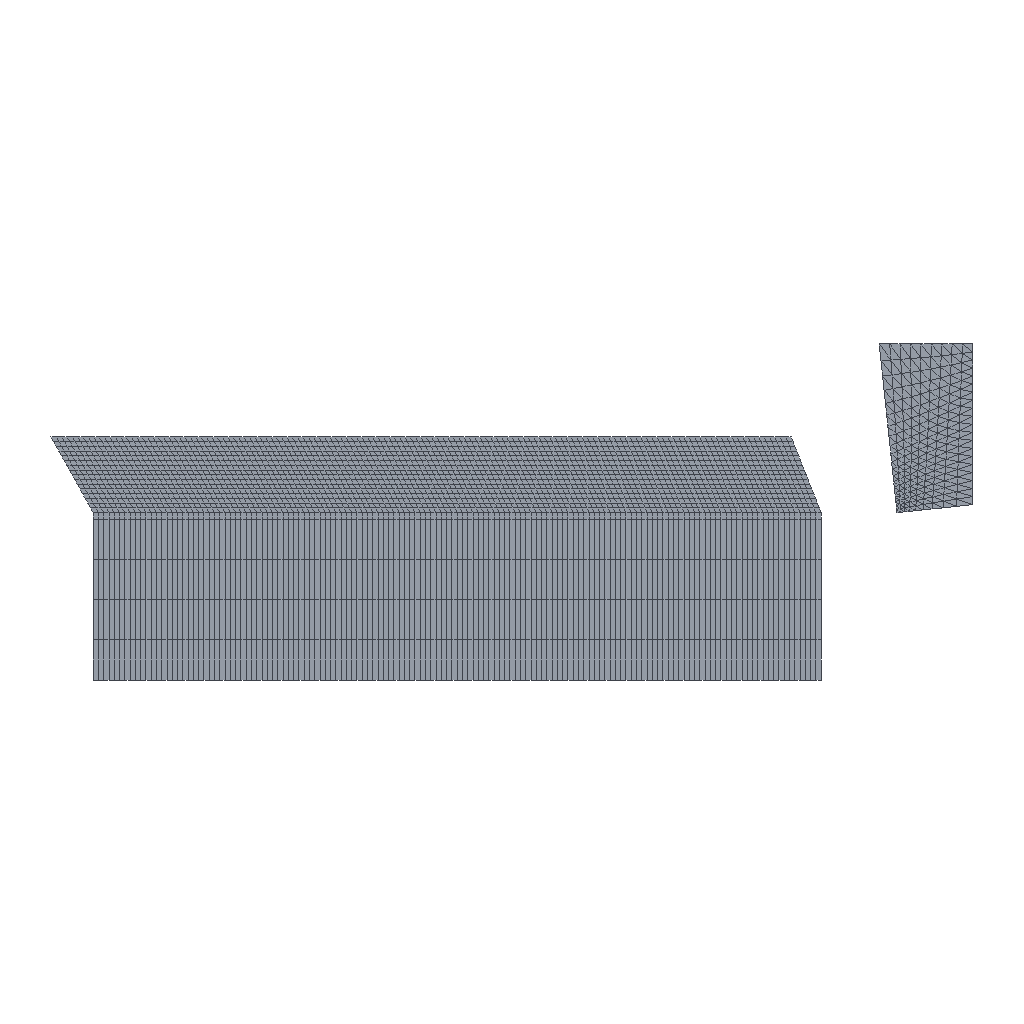Simulation study | abaqus
Set-up summary:
category,name,step,type,value,unit,region
solver,abaqus
solver,version,,,Abaqus/Explicit 2020
units,not stated in the deck,,not stated
analysis,deck,,dynamic temperature-displacement,dynamic temperature-displacement
load_step,Step-1,Step-1,dynamic temperature-displacement
load_step,requested,,,1
mesh,nodes,,,3268
mesh,elements,,,3258
element_type,CPE3T,,plane,360
element_type,CPE4RT,,plane,2898
load,load commands in deck,,count,1
bc,support commands in deck,,count,4
material,TI,,in results
material,TI-COPY,,in results
material,TI6AL4V-GAI,,in results
material,TI6AL4V-SUN,,in results
material,YG6,,in results
check,setup vs results,,match,"per instance, exact: element labels, types and connectivity; labels of the nodes the elements use; coordinates of those nodes at SINGLE_PRECISION in 2 of 2 instance(s)"
Abaqus input file, long lists of numbers shortened:
*Heading
** Job name: Job-4 Model name: Model-1-Copy-Copy2
** Generated by: Abaqus/CAE 2020
*Preprint, echo=NO, model=NO, history=NO, contact=NO
**
** PARTS
**
*Part, name=Part-tool
*Node
      1, 0.05,  0.3
      2, 0.05659,  0.2373
** (208 more lines like these left out)
*Element, type=CPE3T
  1,   1,   2,  23
  2,  23,  22,   1
** (358 more lines like these left out)
*Nset, nset=Set-6, generate
   1,  210,    1
*Elset, elset=Set-6, generate
   1,  360,    1
** Section: Section-tool
*Solid Section, elset=Set-6, material=YG6
2.5,
*End Part
**
*Part, name=work
*Node
      1,   1.217,      -0.8125
      2,   1.217, -0.2125
** (3056 more lines like these left out)
*Element, type=CPE4RT
  1,    1,    9,  593,  288
  2,    9,   10,  594,  593
** (2896 more lines like these left out)
*Nset, nset=Set-4, generate
    1,  3058,     1
*Elset, elset=Set-4, generate
    1,  2898,     1
*Nset, nset=Set-12, generate
    1,  3058,     1
*Elset, elset=Set-12
    1,    2,    3,    4,    5,    6,    7,    8,    9,   10,   11,   12,   13,   14,   15,   16
   17,   18,   19,   20,   21,   22,   23,   24,   25,   26,   27,   28,   29,   30,   31,   32
** (171 more lines like these left out)
*Nset, nset=Set-13
   2,   3,   5,   6,  12,  13,  14,  15,  16,  17,  18,  19,  20,  21,  22,  23
  24,  25,  26,  27,  28,  29,  30,  31,  32,  33,  34,  35,  36,  37,  38,  39
** (16 more lines like these left out)
*Elset, elset=Set-13, generate
 553,  690,    1
** Section: ti
*Solid Section, elset=Set-12, material=ti
,
** Section: middle
*Solid Section, elset=Set-13, material=ti-Copy
,
*End Part
**
**
** ASSEMBLY
**
*Assembly, name=Assembly
**
*Instance, name=Part-tool-1, part=Part-tool
    1.384,     0.1423,           0.
*End Instance
**
*Instance, name=work-1, part=work
*End Instance
**
*Node
      1,   1.784,   0.4423,           0.
*Nset, nset=Set-9, instance=work-1
   3,   4,   6, 149, 150, 151
*Elset, elset=Set-9, instance=work-1
 549, 550, 551, 552, 690
*Nset, nset=Set-10, instance=Part-tool-1, generate
   1,  210,    1
*Elset, elset=Set-10, instance=Part-tool-1, generate
   1,  360,    1
*Nset, nset=Set-11, instance=work-1
   3,   4, 149, 150, 151
*Elset, elset=Set-11, instance=work-1, generate
 549,  552,    1
*Nset, nset=Set-15, instance=work-1
   1,   3,   4, 149, 150, 151, 152, 153, 154, 155, 156, 157, 158, 159, 160, 161
 162, 163, 164, 165, 166, 167, 168, 169, 170, 171, 172, 173, 174, 175, 176, 177
** (7 more lines like these left out)
*Elset, elset=Set-15, instance=work-1
   1,   5,   9,  13,  17,  21,  25,  29,  33,  37,  41,  45,  49,  53,  57,  61
  65,  69,  73,  77,  81,  85,  89,  93,  97, 101, 105, 109, 113, 117, 121, 125
** (7 more lines like these left out)
*Nset, nset=Set-RP
 1,
*Nset, nset=b_Set-7, instance=Part-tool-1, generate
   1,  210,    1
*Elset, elset=b_Set-7, instance=Part-tool-1, generate
   1,  360,    1
*Nset, nset=s_Set-14, instance=work-1
    2,    3,    5,    6,    7,    8,   12,   13,   14,   15,   16,   17,   18,   19,   20,   21
   22,   23,   24,   25,   26,   27,   28,   29,   30,   31,   32,   33,   34,   35,   36,   37
** (155 more lines like these left out)
*Elset, elset=s_Set-14, instance=work-1, generate
  553,  2898,     1
*Nset, nset=_PickedSet38, internal
 1,
*Elset, elset=_Surf-8_S3, internal, instance=work-1
 690,
*Surface, type=ELEMENT, name=Surf-8
_Surf-8_S3, S3
*Elset, elset=_m_Surf-7_S1, internal, instance=Part-tool-1, generate
  1,  39,   2
*Elset, elset=_m_Surf-7_S2, internal, instance=Part-tool-1
   2,  39,  42,  79,  82, 119, 122, 159, 162, 199, 202, 239, 242, 279, 282, 319
 322, 359
*Surface, type=ELEMENT, name=m_Surf-7
_m_Surf-7_S1, S1
_m_Surf-7_S2, S2
*Surface, type=NODE, name=s_Set-14_CNS_, internal
s_Set-14, 1.
** Constraint: Constraint-1
*Rigid Body, ref node=_PickedSet38, elset=b_Set-7, position=CENTER OF MASS
*End Assembly
**
** MATERIALS
**
*Material, name=TI6AL4V-gai
*Conductivity
  5.44, 20.
   6.7,100.
  8.79,200.
 10.47,300.
 12.56,400.
 14.24,500.
 15.49,600.
*Damage Initiation, criterion=JOHNSON COOK
 -0.09,  0.25, -0.48, 0.014,  3.87, 1630.,   25.,    1.
*Damage Evolution, type=DISPLACEMENT
 0.1,
*Density
 4.44e-09,
*Elastic
105000., 0.31
*Expansion
 9.4e-06,100.
 9.5e-06,200.
 9.6e-06,300.
 9.7e-06,400.
 9.9e-06,500.
   1e-05,600.
*Inelastic Heat Fraction
         0.9,
*Plastic, hardening=JOHNSON COOK
875.,  793., 0.386,  0.71, 1630.,   25.
*Rate Dependent, type=JOHNSON COOK
 0.01,1.
*Specific Heat
 5.65e+08, 20.
 6.78e+08,100.
 6.91e+08,200.
 7.03e+08,300.
 7.41e+08,400.
 7.54e+08,500.
 8.79e+08,600.
*Material, name=TI6AL4V-sun
*Conductivity
  5.44, 20.
   6.7,100.
  8.79,200.
 10.47,300.
 12.56,400.
 14.24,500.
 15.49,600.
*Damage Initiation, criterion=JOHNSON COOK
 -0.09,  0.25, -0.48, 0.014,  3.87, 1630.,   25.,    1.
*Damage Evolution, type=DISPLACEMENT
 0.15,
*Density
 4.44e-09,
*Elastic
105000., 0.31
*Expansion
 9.4e-06,100.
 9.5e-06,200.
 9.6e-06,300.
 9.7e-06,400.
 9.9e-06,500.
   1e-05,600.
*Inelastic Heat Fraction
         0.9,
*Plastic, hardening=JOHNSON COOK
875.,  793., 0.386,  0.71, 1630.,   25.
*Rate Dependent, type=JOHNSON COOK
 0.01,1.
*Specific Heat
 5.65e+08, 20.
 6.78e+08,100.
 6.91e+08,200.
 7.03e+08,300.
 7.41e+08,400.
 7.54e+08,500.
 8.79e+08,600.
*Material, name=YG6
*Conductivity
 79.6,
*Density
 1.485e-08,
*Elastic
640000., 0.22
*Expansion
 4.7e-06,
*Inelastic Heat Fraction
         0.9,
*Specific Heat
 1.76e+08,
*Material, name=ti
*Conductivity
  7.5, 20.
  8.7,200.
 11.8,500.
*Damage Initiation, criterion=JOHNSON COOK
 -0.09,  0.25,  -0.5, 0.014,  3.87, 1650.,   25.,    1.
*Damage Evolution, type=DISPLACEMENT
 0.075,
*Density
 4.44e-09,
*Elastic
108000., 0.33
*Expansion
 9.1e-06, 20.
 9.2e-06,250.
 9.7e-06,500.
*Inelastic Heat Fraction
         0.9,
*Plastic, hardening=JOHNSON COOK
860., 683., 0.47,   1.,1650.,  25.
*Rate Dependent, type=JOHNSON COOK
 0.035,1.
*Specific Heat
 5.263e+08,
*Material, name=ti-Copy
*Conductivity
  7.5, 20.
  8.7,200.
 11.8,500.
*Damage Initiation, criterion=JOHNSON COOK
 -0.09,  0.25,  -0.5, 0.014,  3.87, 1650.,   25.,    1.
*Damage Evolution, type=DISPLACEMENT
 0.04,
*Density
 4.44e-09,
*Elastic
108000., 0.33
*Expansion
 9.1e-06, 20.
 9.2e-06,250.
 9.7e-06,500.
*Inelastic Heat Fraction
         0.9,
*Plastic, hardening=JOHNSON COOK
860., 683., 0.47,   1.,1650.,  25.
*Rate Dependent, type=JOHNSON COOK
 0.035,1.
*Specific Heat
 5.263e+08,
**
** INTERACTION PROPERTIES
**
*Surface Interaction, name=IntProp-1
*Friction
 0.1,
*Surface Behavior, pressure-overclosure=HARD
*Surface Interaction, name=zijie
*Friction
 0.5,
*Surface Behavior, pressure-overclosure=HARD
**
** BOUNDARY CONDITIONS
**
** Name: BC-1 Type: 对称/反对称/完全固定
*Boundary
Set-15, ENCASTRE
**
** PREDEFINED FIELDS
**
** Name: Predefined Field-1   Type: Temperature
*Initial Conditions, type=TEMPERATURE
Set-9, 20.
** Name: Predefined Field-2   Type: Temperature
*Initial Conditions, type=TEMPERATURE
Set-10, 20.
** ----------------------------------------------------------------
**
** STEP: Step-1
**
*Step, name=Step-1, nlgeom=YES
*Dynamic Temperature-displacement, Explicit
, 0.001
*Bulk Viscosity
0.06, 1.2
** Mass Scaling: Semi-Automatic
**               Whole Model
*Fixed Mass Scaling, factor=200.
**
** BOUNDARY CONDITIONS
**
** Name: BC-2 Type: 速度/角速度
*Boundary, type=VELOCITY
Set-RP, 1, 1, -1666.
Set-RP, 2, 2
Set-RP, 6, 6
*Adaptive Mesh Controls, name=Ada-1, curvature refinement=5.
0.5, 0., 0.5
**
** INTERACTIONS
**
** Interaction: Int-1
*Contact Pair, interaction=IntProp-1, mechanical constraint=KINEMATIC, cpset=Int-1
m_Surf-7, s_Set-14_CNS_
** Interaction: Int-2
*Contact, op=NEW
*Contact Inclusions, ALL EXTERIOR
*Contact Property Assignment
 ,  , zijie
**
** OUTPUT REQUESTS
**
*Restart, write, number interval=1, time marks=NO
**
** FIELD OUTPUT: F-Output-1
**
*Output, field, number interval=100
*Node Output
A, NT, RF, RFL, U, V
*Element Output, directions=YES
E, EVF, HFL, LE, MISES, PE, PEEQ, PEEQVAVG, PEVAVG, S, STATUS, SVAVG, TEMP
*Contact Output
CSTRESS,
**
** HISTORY OUTPUT: H-Output-1
**
*Output, history, time interval=5e-07
*Node Output, nset=Set-RP
RF1, RF2, RF3
*End Step
Results summary:
result,step,Step-1,completed,increments=65885 time=0.001/0.001
result,analysis,,,"dynamic temperature-displacement, explict"
result,last_loadstep,,,1
result,primary field,,,"U, NT11"
result,reaction total,,FX,-20.931,model units
result,reaction total,,FY,-39.42,model units
result,reaction total,,FZ,0.0,model units